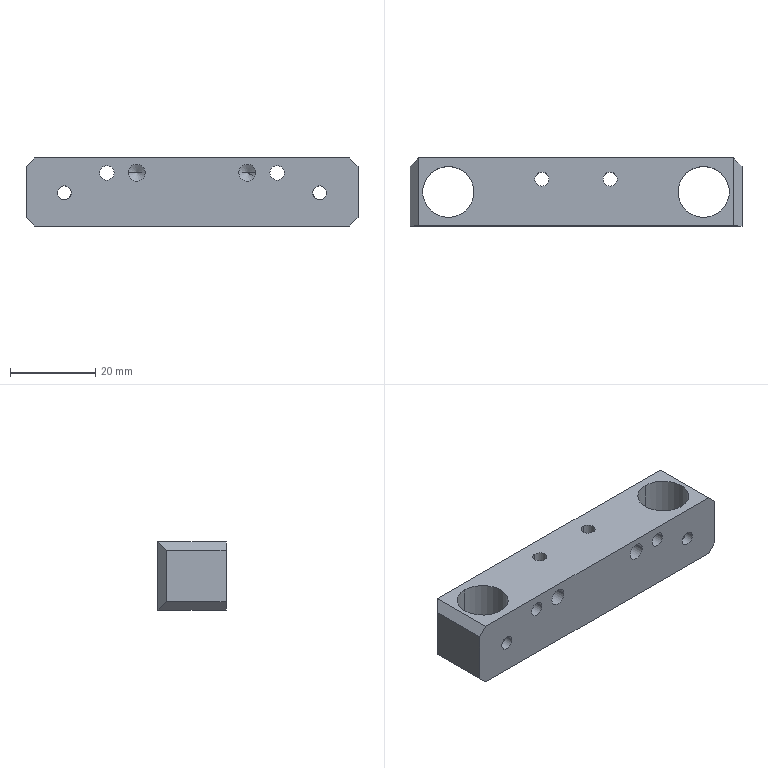NC program | NX | posted with a generic post | part box 78 x 16 x 16 mm
Whole program:
N10 G17 G21 G94 G90
(DRILLING_COPY , TOOL : ZXZ)
N12 T21 M6
N14 G54
N16 G17 G0 G90 X-30. Y0. B0. C0. S3500 M3
N18 G43 Z30. H21
N20 G94 G81 G98 Z-1. F250. R3.
N22 X-8. Y3.
N24 X8.
N26 X30. Y0.
N28 G80
N30 G0 X30. Y0. Z30.
N32 M5
(DRILLING_COPY_1_COPY_COPY , TOOL : 3.3ZT)
N34 T13 M6
N36 G54
N38 G17 G0 G90 X8. Y3. B0. C0. S2000 M3
N40 G43 Z30. H13
N42 G94 G83 G98 Z-17.991 F150. Q2. R3.
N44 X-8.
N46 G80
N48 G0 X-8. Y3. Z30.
N50 M5
(HOLE_MILLING_1 , TOOL : D10)
N52 T04 M6
N54 G54
N56 G17 G0 G90 X-30. Y0. B0. C0. S3500 M3
N58 G43 Z30. H4
N60 Z0.5
N62 G94 G3 X-29.525 Y-0.475 R0.475 F2000.
N64 X-29.05 Y0. R0.475
N66 X-29.05 Y0. Z0.28 I-0.95 J0.
N68 X-29.05 Y0. Z0.06 I-0.95 J0.
N70 X-29.05 Y0. Z-0.16 I-0.95 J0.
N72 X-29.05 Y0. Z-0.38 I-0.95 J0.
N74 X-29.05 Y0. Z-0.6 I-0.95 J0.
N76 X-29.05 Y0. Z-0.82 I-0.95 J0.
N78 X-29.05 Y0. Z-1.04 I-0.95 J0.
N80 X-29.05 Y0. Z-1.26 I-0.95 J0.
N82 X-29.05 Y0. Z-1.48 I-0.95 J0.
N84 X-29.05 Y0. Z-1.7 I-0.95 J0.
N86 X-29.05 Y0. Z-1.92 I-0.95 J0.
N88 X-29.05 Y0. Z-2.14 I-0.95 J0.
N90 X-29.05 Y0. Z-2.36 I-0.95 J0.
N92 X-29.05 Y0. Z-2.58 I-0.95 J0.
N94 X-29.05 Y0. Z-2.8 I-0.95 J0.
N96 X-29.05 Y0. Z-3.02 I-0.95 J0.
N98 X-29.05 Y0. Z-3.24 I-0.95 J0.
N100 X-29.05 Y0. Z-3.46 I-0.95 J0.
N102 X-29.05 Y0. Z-3.68 I-0.95 J0.
N104 X-29.05 Y0. Z-3.9 I-0.95 J0.
N106 X-29.05 Y0. Z-4.12 I-0.95 J0.
N108 X-29.05 Y0. Z-4.34 I-0.95 J0.
N110 X-29.05 Y0. Z-4.56 I-0.95 J0.
N112 X-29.05 Y0. Z-4.78 I-0.95 J0.
N114 X-29.05 Y0. Z-5. I-0.95 J0.
N116 X-29.05 Y0. Z-5.22 I-0.95 J0.
N118 X-29.05 Y0. Z-5.44 I-0.95 J0.
N120 X-29.05 Y0. Z-5.66 I-0.95 J0.
N122 X-29.05 Y0. Z-5.88 I-0.95 J0.
N124 X-29.05 Y0. Z-6.1 I-0.95 J0.
N126 X-29.05 Y0. Z-6.32 I-0.95 J0.
N128 X-29.05 Y0. Z-6.54 I-0.95 J0.
N130 X-29.05 Y0. Z-6.76 I-0.95 J0.
N132 X-29.05 Y0. Z-6.98 I-0.95 J0.
N134 X-29.05 Y0. Z-7.2 I-0.95 J0.
N136 X-29.05 Y0. Z-7.42 I-0.95 J0.
N138 X-29.05 Y0. Z-7.64 I-0.95 J0.
N140 X-29.05 Y0. Z-7.86 I-0.95 J0.
N142 X-29.05 Y0. Z-8.08 I-0.95 J0.
N144 X-29.05 Y0. Z-8.3 I-0.95 J0.
N146 X-29.05 Y0. Z-8.52 I-0.95 J0.
N148 X-29.05 Y0. Z-8.74 I-0.95 J0.
N150 X-29.05 Y0. Z-8.96 I-0.95 J0.
N152 X-29.05 Y0. Z-9.18 I-0.95 J0.
N154 X-29.05 Y0. Z-9.4 I-0.95 J0.
N156 X-29.05 Y0. Z-9.62 I-0.95 J0.
N158 X-29.05 Y0. Z-9.84 I-0.95 J0.
N160 X-29.05 Y0. Z-10.06 I-0.95 J0.
N162 X-29.05 Y0. Z-10.28 I-0.95 J0.
N164 X-29.05 Y0. Z-10.5 I-0.95 J0.
N166 X-29.05 Y0. Z-10.72 I-0.95 J0.
N168 X-29.05 Y0. Z-10.94 I-0.95 J0.
N170 X-29.05 Y0. Z-11.16 I-0.95 J0.
N172 X-29.05 Y0. Z-11.38 I-0.95 J0.
N174 X-29.05 Y0. Z-11.6 I-0.95 J0.
N176 X-29.05 Y0. Z-11.82 I-0.95 J0.
N178 X-29.05 Y0. Z-12.04 I-0.95 J0.
N180 X-29.05 Y0. Z-12.26 I-0.95 J0.
N182 X-29.05 Y0. Z-12.48 I-0.95 J0.
N184 X-29.05 Y0. Z-12.7 I-0.95 J0.
N186 X-29.05 Y0. Z-12.92 I-0.95 J0.
N188 X-29.05 Y0. Z-13.14 I-0.95 J0.
N190 X-29.05 Y0. Z-13.36 I-0.95 J0.
N192 X-29.05 Y0. Z-13.58 I-0.95 J0.
N194 X-29.05 Y0. Z-13.8 I-0.95 J0.
N196 X-29.05 Y0. Z-14.02 I-0.95 J0.
N198 X-29.05 Y0. Z-14.24 I-0.95 J0.
N200 X-29.05 Y0. Z-14.46 I-0.95 J0.
N202 X-29.05 Y0. Z-14.68 I-0.95 J0.
N204 X-29.05 Y0. Z-14.9 I-0.95 J0.
N206 X-29.05 Y0. Z-15.12 I-0.95 J0.
N208 X-29.05 Y0. Z-15.34 I-0.95 J0.
N210 X-29.05 Y0. Z-15.56 I-0.95 J0.
N212 X-29.05 Y0. Z-15.78 I-0.95 J0.
N214 X-29.05 Y0. Z-16. I-0.95 J0.
N216 X-30. Y0.95 R0.95
N218 X-29.05 Y0. R-0.95
N220 X-29.525 Y0.475 R0.475
N222 X-30. Y0. R0.475
N224 G0 Z30.
N226 X30.
N228 Z0.5
N230 G3 X30.475 Y-0.475 R0.475
N232 X30.95 Y0. R0.475
N234 X30.95 Y0. Z0.28 I-0.95 J0.
N236 X30.95 Y0. Z0.06 I-0.95 J0.
N238 X30.95 Y0. Z-0.16 I-0.95 J0.
N240 X30.95 Y0. Z-0.38 I-0.95 J0.
N242 X30.95 Y0. Z-0.6 I-0.95 J0.
N244 X30.95 Y0. Z-0.82 I-0.95 J0.
N246 X30.95 Y0. Z-1.04 I-0.95 J0.
N248 X30.95 Y0. Z-1.26 I-0.95 J0.
N250 X30.95 Y0. Z-1.48 I-0.95 J0.
N252 X30.95 Y0. Z-1.7 I-0.95 J0.
N254 X30.95 Y0. Z-1.92 I-0.95 J0.
N256 X30.95 Y0. Z-2.14 I-0.95 J0.
N258 X30.95 Y0. Z-2.36 I-0.95 J0.
N260 X30.95 Y0. Z-2.58 I-0.95 J0.
N262 X30.95 Y0. Z-2.8 I-0.95 J0.
N264 X30.95 Y0. Z-3.02 I-0.95 J0.
N266 X30.95 Y0. Z-3.24 I-0.95 J0.
N268 X30.95 Y0. Z-3.46 I-0.95 J0.
N270 X30.95 Y0. Z-3.68 I-0.95 J0.
N272 X30.95 Y0. Z-3.9 I-0.95 J0.
N274 X30.95 Y0. Z-4.12 I-0.95 J0.
N276 X30.95 Y0. Z-4.34 I-0.95 J0.
N278 X30.95 Y0. Z-4.56 I-0.95 J0.
N280 X30.95 Y0. Z-4.78 I-0.95 J0.
N282 X30.95 Y0. Z-5. I-0.95 J0.
N284 X30.95 Y0. Z-5.22 I-0.95 J0.
N286 X30.95 Y0. Z-5.44 I-0.95 J0.
N288 X30.95 Y0. Z-5.66 I-0.95 J0.
N290 X30.95 Y0. Z-5.88 I-0.95 J0.
N292 X30.95 Y0. Z-6.1 I-0.95 J0.
N294 X30.95 Y0. Z-6.32 I-0.95 J0.
N296 X30.95 Y0. Z-6.54 I-0.95 J0.
N298 X30.95 Y0. Z-6.76 I-0.95 J0.
N300 X30.95 Y0. Z-6.98 I-0.95 J0.
N302 X30.95 Y0. Z-7.2 I-0.95 J0.
N304 X30.95 Y0. Z-7.42 I-0.95 J0.
N306 X30.95 Y0. Z-7.64 I-0.95 J0.
N308 X30.95 Y0. Z-7.86 I-0.95 J0.
N310 X30.95 Y0. Z-8.08 I-0.95 J0.
N312 X30.95 Y0. Z-8.3 I-0.95 J0.
N314 X30.95 Y0. Z-8.52 I-0.95 J0.
N316 X30.95 Y0. Z-8.74 I-0.95 J0.
N318 X30.95 Y0. Z-8.96 I-0.95 J0.
N320 X30.95 Y0. Z-9.18 I-0.95 J0.
N322 X30.95 Y0. Z-9.4 I-0.95 J0.
N324 X30.95 Y0. Z-9.62 I-0.95 J0.
N326 X30.95 Y0. Z-9.84 I-0.95 J0.
N328 X30.95 Y0. Z-10.06 I-0.95 J0.
N330 X30.95 Y0. Z-10.28 I-0.95 J0.
N332 X30.95 Y0. Z-10.5 I-0.95 J0.
N334 X30.95 Y0. Z-10.72 I-0.95 J0.
N336 X30.95 Y0. Z-10.94 I-0.95 J0.
N338 X30.95 Y0. Z-11.16 I-0.95 J0.
N340 X30.95 Y0. Z-11.38 I-0.95 J0.
N342 X30.95 Y0. Z-11.6 I-0.95 J0.
N344 X30.95 Y0. Z-11.82 I-0.95 J0.
N346 X30.95 Y0. Z-12.04 I-0.95 J0.
N348 X30.95 Y0. Z-12.26 I-0.95 J0.
N350 X30.95 Y0. Z-12.48 I-0.95 J0.
N352 X30.95 Y0. Z-12.7 I-0.95 J0.
N354 X30.95 Y0. Z-12.92 I-0.95 J0.
N356 X30.95 Y0. Z-13.14 I-0.95 J0.
N358 X30.95 Y0. Z-13.36 I-0.95 J0.
N360 X30.95 Y0. Z-13.58 I-0.95 J0.
N362 X30.95 Y0. Z-13.8 I-0.95 J0.
N364 X30.95 Y0. Z-14.02 I-0.95 J0.
N366 X30.95 Y0. Z-14.24 I-0.95 J0.
N368 X30.95 Y0. Z-14.46 I-0.95 J0.
N370 X30.95 Y0. Z-14.68 I-0.95 J0.
N372 X30.95 Y0. Z-14.9 I-0.95 J0.
N374 X30.95 Y0. Z-15.12 I-0.95 J0.
N376 X30.95 Y0. Z-15.34 I-0.95 J0.
N378 X30.95 Y0. Z-15.56 I-0.95 J0.
N380 X30.95 Y0. Z-15.78 I-0.95 J0.
N382 X30.95 Y0. Z-16. I-0.95 J0.
N384 X30. Y0.95 R0.95
N386 X30.95 Y0. R-0.95
N388 X30.475 Y0.475 R0.475
N390 X30. Y0. R0.475
N392 G0 Z30.
N394 M5
(刀补14 , TOOL : D10JING)
N396 T14 M6
N398 G54
N400 G17 G0 G90 X-30. Y0. B0. C0. S3500 M3
N402 G43 Z30. H14
N404 Z0.5
N406 G41 G94 G1 X-29.997 Y-0.1 F2000. D14
N408 G3 X-29.04 Y0. R0.484
N410 X-29.04 Y0. Z-1.5 I-0.96 J0.
N412 X-29.04 Y0. Z-3.5 I-0.96 J0.
N414 X-29.04 Y0. Z-5.5 I-0.96 J0.
N416 X-29.04 Y0. Z-7.5 I-0.96 J0.
N418 X-29.04 Y0. Z-9.5 I-0.96 J0.
N420 X-29.04 Y0. Z-11.5 I-0.96 J0.
N422 X-29.04 Y0. Z-13.5 I-0.96 J0.
N424 X-29.04 Y0. Z-15.5 I-0.96 J0.
N426 X-30. Y0.96 Z-16. R0.96
N428 X-30.96 Y0. R0.96
N430 X-30. Y0.96 R-0.96
N432 X-30.1 Y0.003 R0.484
N434 G40
N436 G1 X-30. Y0.
N438 G0 Z30.
N440 X30.
N442 Z0.5
N444 G41 G1 X30.003 Y-0.1
N446 G3 X30.96 Y0. R0.484
N448 X30.96 Y0. Z-1.5 I-0.96 J0.
N450 X30.96 Y0. Z-3.5 I-0.96 J0.
N452 X30.96 Y0. Z-5.5 I-0.96 J0.
N454 X30.96 Y0. Z-7.5 I-0.96 J0.
N456 X30.96 Y0. Z-9.5 I-0.96 J0.
N458 X30.96 Y0. Z-11.5 I-0.96 J0.
N460 X30.96 Y0. Z-13.5 I-0.96 J0.
N462 X30.96 Y0. Z-15.5 I-0.96 J0.
N464 X30. Y0.96 Z-16. R0.96
N466 X29.04 Y0. R0.96
N468 X30. Y0.96 R-0.96
N470 X29.9 Y0.003 R0.484
N472 G40
N474 G1 X30. Y0.
N476 G0 Z30.
N478 M5
N480 M2